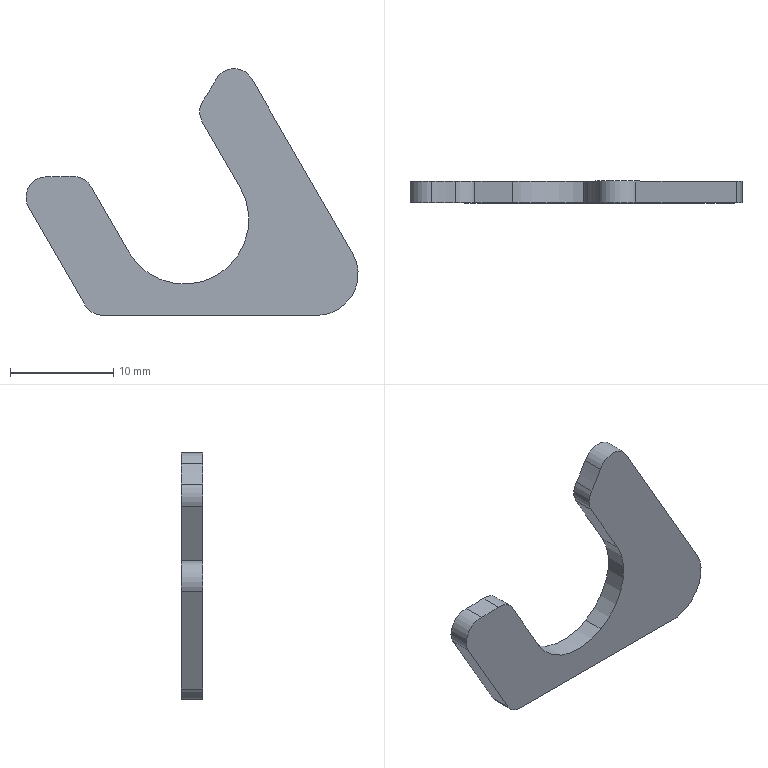Part | SolidWorks | features BaseBody 1 | 1 solid | 18 faces | box 32.238 x 2.1 x 23.947 mm | volume 666.378 mm3 | cylinder 11 | plane 7 | commonest cylinder face diameters 4 x5 8 x2 12.5 x2 35 x2
STEP:
#1=CARTESIAN_POINT('',(182.361,160.,-32.991));
#2=VERTEX_POINT('',#1);
#3=CARTESIAN_POINT('',(183.825,160.,-27.527));
#4=VERTEX_POINT('',#3);
#5=CARTESIAN_POINT('',(180.361,160.,-29.527));
#6=DIRECTION('',(0.,-1.,0.));
#7=DIRECTION('',(0.5,0.,-0.866));
#8=AXIS2_PLACEMENT_3D('',#5,#6,#7);
#9=CIRCLE('',#8,4.);
#10=EDGE_CURVE('',#2,#4,#9,.T.);
#11=ORIENTED_EDGE('',*,*,#10,.F.);
#12=CARTESIAN_POINT('',(182.361,162.1,-32.991));
#13=VERTEX_POINT('',#12);
#14=CARTESIAN_POINT('',(182.361,160.,-32.991));
#15=DIRECTION('',(0.,1.,0.));
#16=VECTOR('',#15,1000.);
#17=LINE('',#14,#16);
#18=EDGE_CURVE('',#2,#13,#17,.T.);
#19=ORIENTED_EDGE('',*,*,#18,.T.);
#20=CARTESIAN_POINT('',(183.825,162.1,-27.527));
#21=VERTEX_POINT('',#20);
#22=CARTESIAN_POINT('',(180.361,162.1,-29.527));
#23=DIRECTION('',(0.,-1.,0.));
#24=DIRECTION('',(0.5,0.,-0.866));
#25=AXIS2_PLACEMENT_3D('',#22,#23,#24);
#26=CIRCLE('',#25,4.);
#27=EDGE_CURVE('',#13,#21,#26,.T.);
#28=ORIENTED_EDGE('',*,*,#27,.T.);
#29=CARTESIAN_POINT('',(183.825,160.,-27.527));
#30=DIRECTION('',(0.,1.,0.));
#31=VECTOR('',#30,1000.);
#32=LINE('',#29,#31);
#33=EDGE_CURVE('',#4,#21,#32,.T.);
#34=ORIENTED_EDGE('',*,*,#33,.F.);
#35=EDGE_LOOP('',(#11,#19,#28,#34));
#36=FACE_OUTER_BOUND('',#35,.T.);
#37=CARTESIAN_POINT('',(180.361,160.,-29.527));
#38=DIRECTION('',(0.,1.,0.));
#39=DIRECTION('',(0.5,0.,-0.866));
#40=AXIS2_PLACEMENT_3D('',#37,#38,#39);
#41=CYLINDRICAL_SURFACE('',#40,4.);
#42=ADVANCED_FACE('',(#36),#41,.T.);
#43=CARTESIAN_POINT('',(170.625,160.,-29.663));
#44=VERTEX_POINT('',#43);
#45=CARTESIAN_POINT('',(162.087,160.,-27.375));
#46=VERTEX_POINT('',#45);
#47=CARTESIAN_POINT('',(167.5,160.,-24.25));
#48=DIRECTION('',(0.,1.,0.));
#49=DIRECTION('',(-0.5,0.,0.866));
#50=AXIS2_PLACEMENT_3D('',#47,#48,#49);
#51=CIRCLE('',#50,6.25);
#52=EDGE_CURVE('',#44,#46,#51,.T.);
#53=ORIENTED_EDGE('',*,*,#52,.F.);
#54=CARTESIAN_POINT('',(170.625,162.1,-29.663));
#55=VERTEX_POINT('',#54);
#56=CARTESIAN_POINT('',(170.625,160.,-29.663));
#57=DIRECTION('',(0.,1.,0.));
#58=VECTOR('',#57,1000.);
#59=LINE('',#56,#58);
#60=EDGE_CURVE('',#44,#55,#59,.T.);
#61=ORIENTED_EDGE('',*,*,#60,.T.);
#62=CARTESIAN_POINT('',(162.087,162.1,-27.375));
#63=VERTEX_POINT('',#62);
#64=CARTESIAN_POINT('',(167.5,162.1,-24.25));
#65=DIRECTION('',(0.,1.,0.));
#66=DIRECTION('',(-0.5,0.,0.866));
#67=AXIS2_PLACEMENT_3D('',#64,#65,#66);
#68=CIRCLE('',#67,6.25);
#69=EDGE_CURVE('',#55,#63,#68,.T.);
#70=ORIENTED_EDGE('',*,*,#69,.T.);
#71=CARTESIAN_POINT('',(162.087,160.,-27.375));
#72=DIRECTION('',(0.,1.,0.));
#73=VECTOR('',#72,1000.);
#74=LINE('',#71,#73);
#75=EDGE_CURVE('',#46,#63,#74,.T.);
#76=ORIENTED_EDGE('',*,*,#75,.F.);
#77=EDGE_LOOP('',(#53,#61,#70,#76));
#78=FACE_OUTER_BOUND('',#77,.T.);
#79=CARTESIAN_POINT('',(167.5,160.,-24.25));
#80=DIRECTION('',(0.,1.,0.));
#81=DIRECTION('',(0.5,0.,-0.866));
#82=AXIS2_PLACEMENT_3D('',#79,#80,#81);
#83=CYLINDRICAL_SURFACE('',#82,6.25);
#84=ADVANCED_FACE('',(#78),#83,.F.);
#85=ORIENTED_EDGE('',*,*,#60,.F.);
#86=CARTESIAN_POINT('',(172.913,160.,-21.125));
#87=VERTEX_POINT('',#86);
#88=CARTESIAN_POINT('',(167.5,160.,-24.25));
#89=DIRECTION('',(0.,1.,0.));
#90=DIRECTION('',(-0.5,0.,0.866));
#91=AXIS2_PLACEMENT_3D('',#88,#89,#90);
#92=CIRCLE('',#91,6.25);
#93=EDGE_CURVE('',#87,#44,#92,.T.);
#94=ORIENTED_EDGE('',*,*,#93,.F.);
#95=CARTESIAN_POINT('',(172.913,162.1,-21.125));
#96=VERTEX_POINT('',#95);
#97=CARTESIAN_POINT('',(172.913,160.,-21.125));
#98=DIRECTION('',(0.,1.,0.));
#99=VECTOR('',#98,1000.);
#100=LINE('',#97,#99);
#101=EDGE_CURVE('',#87,#96,#100,.T.);
#102=ORIENTED_EDGE('',*,*,#101,.T.);
#103=CARTESIAN_POINT('',(167.5,162.1,-24.25));
#104=DIRECTION('',(0.,1.,0.));
#105=DIRECTION('',(-0.5,0.,0.866));
#106=AXIS2_PLACEMENT_3D('',#103,#104,#105);
#107=CIRCLE('',#106,6.25);
#108=EDGE_CURVE('',#96,#55,#107,.T.);
#109=ORIENTED_EDGE('',*,*,#108,.T.);
#110=EDGE_LOOP('',(#85,#94,#102,#109));
#111=FACE_OUTER_BOUND('',#110,.T.);
#112=CARTESIAN_POINT('',(167.5,160.,-24.25));
#113=DIRECTION('',(0.,1.,0.));
#114=DIRECTION('',(0.5,0.,-0.866));
#115=AXIS2_PLACEMENT_3D('',#112,#113,#114);
#116=CYLINDRICAL_SURFACE('',#115,6.25);
#117=ADVANCED_FACE('',(#111),#116,.F.);
#118=CARTESIAN_POINT('',(158.422,162.1,-21.026));
#119=VERTEX_POINT('',#118);
#120=CARTESIAN_POINT('',(162.087,162.1,-27.375));
#121=DIRECTION('',(-0.5,0.,0.866));
#122=VECTOR('',#121,1000.);
#123=LINE('',#120,#122);
#124=EDGE_CURVE('',#63,#119,#123,.T.);
#125=ORIENTED_EDGE('',*,*,#124,.T.);
#126=CARTESIAN_POINT('',(158.422,160.,-21.026));
#127=VERTEX_POINT('',#126);
#128=CARTESIAN_POINT('',(158.422,160.,-21.026));
#129=DIRECTION('',(0.,1.,0.));
#130=VECTOR('',#129,1000.);
#131=LINE('',#128,#130);
#132=EDGE_CURVE('',#127,#119,#131,.T.);
#133=ORIENTED_EDGE('',*,*,#132,.F.);
#134=CARTESIAN_POINT('',(162.087,160.,-27.375));
#135=DIRECTION('',(-0.5,0.,0.866));
#136=VECTOR('',#135,1000.);
#137=LINE('',#134,#136);
#138=EDGE_CURVE('',#46,#127,#137,.T.);
#139=ORIENTED_EDGE('',*,*,#138,.F.);
#140=ORIENTED_EDGE('',*,*,#75,.T.);
#141=EDGE_LOOP('',(#125,#133,#139,#140));
#142=FACE_OUTER_BOUND('',#141,.T.);
#143=CARTESIAN_POINT('',(162.087,160.,-27.375));
#144=DIRECTION('',(-0.866,0.,-0.5));
#145=DIRECTION('',(0.5,0.,-0.866));
#146=AXIS2_PLACEMENT_3D('',#143,#144,#145);
#147=PLANE('',#146);
#148=ADVANCED_FACE('',(#142),#147,.F.);
#149=CARTESIAN_POINT('',(156.516,162.1,-20.033));
#150=VERTEX_POINT('',#149);
#151=CARTESIAN_POINT('',(156.69,162.1,-22.026));
#152=DIRECTION('',(0.,-1.,0.));
#153=DIRECTION('',(-0.5,0.,0.866));
#154=AXIS2_PLACEMENT_3D('',#151,#152,#153);
#155=CIRCLE('',#154,2.);
#156=EDGE_CURVE('',#119,#150,#155,.T.);
#157=ORIENTED_EDGE('',*,*,#156,.T.);
#158=CARTESIAN_POINT('',(156.516,160.,-20.033));
#159=VERTEX_POINT('',#158);
#160=CARTESIAN_POINT('',(156.516,160.,-20.033));
#161=DIRECTION('',(0.,1.,0.));
#162=VECTOR('',#161,1000.);
#163=LINE('',#160,#162);
#164=EDGE_CURVE('',#159,#150,#163,.T.);
#165=ORIENTED_EDGE('',*,*,#164,.F.);
#166=CARTESIAN_POINT('',(156.69,160.,-22.026));
#167=DIRECTION('',(0.,-1.,0.));
#168=DIRECTION('',(-0.5,0.,0.866));
#169=AXIS2_PLACEMENT_3D('',#166,#167,#168);
#170=CIRCLE('',#169,2.);
#171=EDGE_CURVE('',#127,#159,#170,.T.);
#172=ORIENTED_EDGE('',*,*,#171,.F.);
#173=ORIENTED_EDGE('',*,*,#132,.T.);
#174=EDGE_LOOP('',(#157,#165,#172,#173));
#175=FACE_OUTER_BOUND('',#174,.T.);
#176=CARTESIAN_POINT('',(156.69,160.,-22.026));
#177=DIRECTION('',(0.,1.,0.));
#178=DIRECTION('',(0.5,0.,-0.866));
#179=AXIS2_PLACEMENT_3D('',#176,#177,#178);
#180=CYLINDRICAL_SURFACE('',#179,2.);
#181=ADVANCED_FACE('',(#175),#180,.T.);
#182=CARTESIAN_POINT('',(154.213,162.1,-20.081));
#183=VERTEX_POINT('',#182);
#184=CARTESIAN_POINT('',(155.,162.1,-2.599));
#185=DIRECTION('',(0.,1.,0.));
#186=DIRECTION('',(-0.5,0.,0.866));
#187=AXIS2_PLACEMENT_3D('',#184,#185,#186);
#188=CIRCLE('',#187,17.5);
#189=EDGE_CURVE('',#150,#183,#188,.T.);
#190=ORIENTED_EDGE('',*,*,#189,.T.);
#191=CARTESIAN_POINT('',(154.213,160.,-20.081));
#192=VERTEX_POINT('',#191);
#193=CARTESIAN_POINT('',(154.213,160.,-20.081));
#194=DIRECTION('',(0.,1.,0.));
#195=VECTOR('',#194,1000.);
#196=LINE('',#193,#195);
#197=EDGE_CURVE('',#192,#183,#196,.T.);
#198=ORIENTED_EDGE('',*,*,#197,.F.);
#199=CARTESIAN_POINT('',(155.,160.,-2.599));
#200=DIRECTION('',(0.,1.,0.));
#201=DIRECTION('',(-0.5,0.,0.866));
#202=AXIS2_PLACEMENT_3D('',#199,#200,#201);
#203=CIRCLE('',#202,17.5);
#204=EDGE_CURVE('',#159,#192,#203,.T.);
#205=ORIENTED_EDGE('',*,*,#204,.F.);
#206=ORIENTED_EDGE('',*,*,#164,.T.);
#207=EDGE_LOOP('',(#190,#198,#205,#206));
#208=FACE_OUTER_BOUND('',#207,.T.);
#209=CARTESIAN_POINT('',(155.,160.,-2.599));
#210=DIRECTION('',(0.,1.,0.));
#211=DIRECTION('',(0.5,0.,-0.866));
#212=AXIS2_PLACEMENT_3D('',#209,#210,#211);
#213=CYLINDRICAL_SURFACE('',#212,17.5);
#214=ADVANCED_FACE('',(#208),#213,.F.);
#215=CARTESIAN_POINT('',(152.391,162.1,-23.079));
#216=VERTEX_POINT('',#215);
#217=CARTESIAN_POINT('',(154.123,162.1,-22.079));
#218=DIRECTION('',(0.,-1.,0.));
#219=DIRECTION('',(0.5,0.,-0.866));
#220=AXIS2_PLACEMENT_3D('',#217,#218,#219);
#221=CIRCLE('',#220,2.);
#222=EDGE_CURVE('',#183,#216,#221,.T.);
#223=ORIENTED_EDGE('',*,*,#222,.T.);
#224=CARTESIAN_POINT('',(152.391,160.,-23.079));
#225=VERTEX_POINT('',#224);
#226=CARTESIAN_POINT('',(152.391,160.,-23.079));
#227=DIRECTION('',(0.,1.,0.));
#228=VECTOR('',#227,1000.);
#229=LINE('',#226,#228);
#230=EDGE_CURVE('',#225,#216,#229,.T.);
#231=ORIENTED_EDGE('',*,*,#230,.F.);
#232=CARTESIAN_POINT('',(154.123,160.,-22.079));
#233=DIRECTION('',(0.,-1.,0.));
#234=DIRECTION('',(0.5,0.,-0.866));
#235=AXIS2_PLACEMENT_3D('',#232,#233,#234);
#236=CIRCLE('',#235,2.);
#237=EDGE_CURVE('',#192,#225,#236,.T.);
#238=ORIENTED_EDGE('',*,*,#237,.F.);
#239=ORIENTED_EDGE('',*,*,#197,.T.);
#240=EDGE_LOOP('',(#223,#231,#238,#239));
#241=FACE_OUTER_BOUND('',#240,.T.);
#242=CARTESIAN_POINT('',(154.123,160.,-22.079));
#243=DIRECTION('',(0.,1.,0.));
#244=DIRECTION('',(0.5,0.,-0.866));
#245=AXIS2_PLACEMENT_3D('',#242,#243,#244);
#246=CYLINDRICAL_SURFACE('',#245,2.);
#247=ADVANCED_FACE('',(#241),#246,.T.);
#248=CARTESIAN_POINT('',(157.844,162.1,-32.526));
#249=VERTEX_POINT('',#248);
#250=CARTESIAN_POINT('',(157.844,162.1,-32.526));
#251=DIRECTION('',(0.5,0.,-0.866));
#252=VECTOR('',#251,1000.);
#253=LINE('',#250,#252);
#254=EDGE_CURVE('',#216,#249,#253,.T.);
#255=ORIENTED_EDGE('',*,*,#254,.T.);
#256=CARTESIAN_POINT('',(157.844,160.,-32.526));
#257=VERTEX_POINT('',#256);
#258=CARTESIAN_POINT('',(157.844,160.,-32.526));
#259=DIRECTION('',(0.,1.,0.));
#260=VECTOR('',#259,1000.);
#261=LINE('',#258,#260);
#262=EDGE_CURVE('',#257,#249,#261,.T.);
#263=ORIENTED_EDGE('',*,*,#262,.F.);
#264=CARTESIAN_POINT('',(157.844,160.,-32.526));
#265=DIRECTION('',(0.5,0.,-0.866));
#266=VECTOR('',#265,1000.);
#267=LINE('',#264,#266);
#268=EDGE_CURVE('',#225,#257,#267,.T.);
#269=ORIENTED_EDGE('',*,*,#268,.F.);
#270=ORIENTED_EDGE('',*,*,#230,.T.);
#271=EDGE_LOOP('',(#255,#263,#269,#270));
#272=FACE_OUTER_BOUND('',#271,.T.);
#273=CARTESIAN_POINT('',(157.844,160.,-32.526));
#274=DIRECTION('',(0.866,0.,0.5));
#275=DIRECTION('',(-0.5,0.,0.866));
#276=AXIS2_PLACEMENT_3D('',#273,#274,#275);
#277=PLANE('',#276);
#278=ADVANCED_FACE('',(#272),#277,.F.);
#279=CARTESIAN_POINT('',(159.576,162.1,-33.526));
#280=VERTEX_POINT('',#279);
#281=CARTESIAN_POINT('',(159.576,162.1,-31.526));
#282=DIRECTION('',(0.,-1.,0.));
#283=DIRECTION('',(0.5,0.,-0.866));
#284=AXIS2_PLACEMENT_3D('',#281,#282,#283);
#285=CIRCLE('',#284,2.);
#286=EDGE_CURVE('',#249,#280,#285,.T.);
#287=ORIENTED_EDGE('',*,*,#286,.T.);
#288=CARTESIAN_POINT('',(159.576,160.,-33.526));
#289=VERTEX_POINT('',#288);
#290=CARTESIAN_POINT('',(159.576,160.,-33.526));
#291=DIRECTION('',(0.,1.,0.));
#292=VECTOR('',#291,1000.);
#293=LINE('',#290,#292);
#294=EDGE_CURVE('',#289,#280,#293,.T.);
#295=ORIENTED_EDGE('',*,*,#294,.F.);
#296=CARTESIAN_POINT('',(159.576,160.,-31.526));
#297=DIRECTION('',(0.,-1.,0.));
#298=DIRECTION('',(0.5,0.,-0.866));
#299=AXIS2_PLACEMENT_3D('',#296,#297,#298);
#300=CIRCLE('',#299,2.);
#301=EDGE_CURVE('',#257,#289,#300,.T.);
#302=ORIENTED_EDGE('',*,*,#301,.F.);
#303=ORIENTED_EDGE('',*,*,#262,.T.);
#304=EDGE_LOOP('',(#287,#295,#302,#303));
#305=FACE_OUTER_BOUND('',#304,.T.);
#306=CARTESIAN_POINT('',(159.576,160.,-31.526));
#307=DIRECTION('',(0.,1.,0.));
#308=DIRECTION('',(0.5,0.,-0.866));
#309=AXIS2_PLACEMENT_3D('',#306,#307,#308);
#310=CYLINDRICAL_SURFACE('',#309,2.);
#311=ADVANCED_FACE('',(#305),#310,.T.);
#312=CARTESIAN_POINT('',(180.361,162.1,-33.527));
#313=VERTEX_POINT('',#312);
#314=CARTESIAN_POINT('',(159.576,162.1,-33.526));
#315=DIRECTION('',(1.,0.,-0.00002301));
#316=VECTOR('',#315,1000.);
#317=LINE('',#314,#316);
#318=EDGE_CURVE('',#280,#313,#317,.T.);
#319=ORIENTED_EDGE('',*,*,#318,.T.);
#320=CARTESIAN_POINT('',(180.361,160.,-33.527));
#321=VERTEX_POINT('',#320);
#322=CARTESIAN_POINT('',(180.361,160.,-33.527));
#323=DIRECTION('',(0.,1.,0.));
#324=VECTOR('',#323,1000.);
#325=LINE('',#322,#324);
#326=EDGE_CURVE('',#321,#313,#325,.T.);
#327=ORIENTED_EDGE('',*,*,#326,.F.);
#328=CARTESIAN_POINT('',(159.576,160.,-33.526));
#329=DIRECTION('',(1.,0.,-0.00002301));
#330=VECTOR('',#329,1000.);
#331=LINE('',#328,#330);
#332=EDGE_CURVE('',#289,#321,#331,.T.);
#333=ORIENTED_EDGE('',*,*,#332,.F.);
#334=ORIENTED_EDGE('',*,*,#294,.T.);
#335=EDGE_LOOP('',(#319,#327,#333,#334));
#336=FACE_OUTER_BOUND('',#335,.T.);
#337=CARTESIAN_POINT('',(159.576,160.,-33.526));
#338=DIRECTION('',(0.00002301,0.,1.));
#339=DIRECTION('',(-1.,0.,0.00002301));
#340=AXIS2_PLACEMENT_3D('',#337,#338,#339);
#341=PLANE('',#340);
#342=ADVANCED_FACE('',(#336),#341,.F.);
#343=ORIENTED_EDGE('',*,*,#18,.F.);
#344=CARTESIAN_POINT('',(180.361,160.,-29.527));
#345=DIRECTION('',(0.,-1.,0.));
#346=DIRECTION('',(0.5,0.,-0.866));
#347=AXIS2_PLACEMENT_3D('',#344,#345,#346);
#348=CIRCLE('',#347,4.);
#349=EDGE_CURVE('',#321,#2,#348,.T.);
#350=ORIENTED_EDGE('',*,*,#349,.F.);
#351=ORIENTED_EDGE('',*,*,#326,.T.);
#352=CARTESIAN_POINT('',(180.361,162.1,-29.527));
#353=DIRECTION('',(0.,-1.,0.));
#354=DIRECTION('',(0.5,0.,-0.866));
#355=AXIS2_PLACEMENT_3D('',#352,#353,#354);
#356=CIRCLE('',#355,4.);
#357=EDGE_CURVE('',#313,#13,#356,.T.);
#358=ORIENTED_EDGE('',*,*,#357,.T.);
#359=EDGE_LOOP('',(#343,#350,#351,#358));
#360=FACE_OUTER_BOUND('',#359,.T.);
#361=CARTESIAN_POINT('',(180.361,160.,-29.527));
#362=DIRECTION('',(0.,1.,0.));
#363=DIRECTION('',(0.5,0.,-0.866));
#364=AXIS2_PLACEMENT_3D('',#361,#362,#363);
#365=CYLINDRICAL_SURFACE('',#364,4.);
#366=ADVANCED_FACE('',(#360),#365,.T.);
#367=CARTESIAN_POINT('',(174.041,162.1,-10.58));
#368=VERTEX_POINT('',#367);
#369=CARTESIAN_POINT('',(183.825,162.1,-27.527));
#370=DIRECTION('',(-0.5,0.,0.866));
#371=VECTOR('',#370,1000.);
#372=LINE('',#369,#371);
#373=EDGE_CURVE('',#21,#368,#372,.T.);
#374=ORIENTED_EDGE('',*,*,#373,.T.);
#375=CARTESIAN_POINT('',(174.041,160.,-10.58));
#376=VERTEX_POINT('',#375);
#377=CARTESIAN_POINT('',(174.041,160.,-10.58));
#378=DIRECTION('',(0.,1.,0.));
#379=VECTOR('',#378,1000.);
#380=LINE('',#377,#379);
#381=EDGE_CURVE('',#376,#368,#380,.T.);
#382=ORIENTED_EDGE('',*,*,#381,.F.);
#383=CARTESIAN_POINT('',(183.825,160.,-27.527));
#384=DIRECTION('',(-0.5,0.,0.866));
#385=VECTOR('',#384,1000.);
#386=LINE('',#383,#385);
#387=EDGE_CURVE('',#4,#376,#386,.T.);
#388=ORIENTED_EDGE('',*,*,#387,.F.);
#389=ORIENTED_EDGE('',*,*,#33,.T.);
#390=EDGE_LOOP('',(#374,#382,#388,#389));
#391=FACE_OUTER_BOUND('',#390,.T.);
#392=CARTESIAN_POINT('',(183.825,160.,-27.527));
#393=DIRECTION('',(-0.866,0.,-0.5));
#394=DIRECTION('',(0.5,0.,-0.866));
#395=AXIS2_PLACEMENT_3D('',#392,#393,#394);
#396=PLANE('',#395);
#397=ADVANCED_FACE('',(#391),#396,.F.);
#398=CARTESIAN_POINT('',(170.534,162.1,-10.659));
#399=VERTEX_POINT('',#398);
#400=CARTESIAN_POINT('',(172.309,162.1,-11.58));
#401=DIRECTION('',(0.,-1.,0.));
#402=DIRECTION('',(-0.5,0.,0.866));
#403=AXIS2_PLACEMENT_3D('',#400,#401,#402);
#404=CIRCLE('',#403,2.);
#405=EDGE_CURVE('',#368,#399,#404,.T.);
#406=ORIENTED_EDGE('',*,*,#405,.T.);
#407=CARTESIAN_POINT('',(170.534,160.,-10.659));
#408=VERTEX_POINT('',#407);
#409=CARTESIAN_POINT('',(170.534,160.,-10.659));
#410=DIRECTION('',(0.,1.,0.));
#411=VECTOR('',#410,1000.);
#412=LINE('',#409,#411);
#413=EDGE_CURVE('',#408,#399,#412,.T.);
#414=ORIENTED_EDGE('',*,*,#413,.F.);
#415=CARTESIAN_POINT('',(172.309,160.,-11.58));
#416=DIRECTION('',(0.,-1.,0.));
#417=DIRECTION('',(-0.5,0.,0.866));
#418=AXIS2_PLACEMENT_3D('',#415,#416,#417);
#419=CIRCLE('',#418,2.);
#420=EDGE_CURVE('',#376,#408,#419,.T.);
#421=ORIENTED_EDGE('',*,*,#420,.F.);
#422=ORIENTED_EDGE('',*,*,#381,.T.);
#423=EDGE_LOOP('',(#406,#414,#421,#422));
#424=FACE_OUTER_BOUND('',#423,.T.);
#425=CARTESIAN_POINT('',(172.309,160.,-11.58));
#426=DIRECTION('',(0.,1.,0.));
#427=DIRECTION('',(0.5,0.,-0.866));
#428=AXIS2_PLACEMENT_3D('',#425,#426,#427);
#429=CYLINDRICAL_SURFACE('',#428,2.);
#430=ADVANCED_FACE('',(#424),#429,.T.);
#431=CARTESIAN_POINT('',(169.341,162.1,-12.63));
#432=VERTEX_POINT('',#431);
#433=CARTESIAN_POINT('',(155.,162.1,-2.599));
#434=DIRECTION('',(0.,1.,0.));
#435=DIRECTION('',(-0.5,0.,0.866));
#436=AXIS2_PLACEMENT_3D('',#433,#434,#435);
#437=CIRCLE('',#436,17.5);
#438=EDGE_CURVE('',#399,#432,#437,.T.);
#439=ORIENTED_EDGE('',*,*,#438,.T.);
#440=CARTESIAN_POINT('',(169.341,160.,-12.63));
#441=VERTEX_POINT('',#440);
#442=CARTESIAN_POINT('',(169.341,160.,-12.63));
#443=DIRECTION('',(0.,1.,0.));
#444=VECTOR('',#443,1000.);
#445=LINE('',#442,#444);
#446=EDGE_CURVE('',#441,#432,#445,.T.);
#447=ORIENTED_EDGE('',*,*,#446,.F.);
#448=CARTESIAN_POINT('',(155.,160.,-2.599));
#449=DIRECTION('',(0.,1.,0.));
#450=DIRECTION('',(-0.5,0.,0.866));
#451=AXIS2_PLACEMENT_3D('',#448,#449,#450);
#452=CIRCLE('',#451,17.5);
#453=EDGE_CURVE('',#408,#441,#452,.T.);
#454=ORIENTED_EDGE('',*,*,#453,.F.);
#455=ORIENTED_EDGE('',*,*,#413,.T.);
#456=EDGE_LOOP('',(#439,#447,#454,#455));
#457=FACE_OUTER_BOUND('',#456,.T.);
#458=CARTESIAN_POINT('',(155.,160.,-2.599));
#459=DIRECTION('',(0.,1.,0.));
#460=DIRECTION('',(0.5,0.,-0.866));
#461=AXIS2_PLACEMENT_3D('',#458,#459,#460);
#462=CYLINDRICAL_SURFACE('',#461,17.5);
#463=ADVANCED_FACE('',(#457),#462,.F.);
#464=CARTESIAN_POINT('',(169.247,162.1,-14.776));
#465=VERTEX_POINT('',#464);
#466=CARTESIAN_POINT('',(170.979,162.1,-13.776));
#467=DIRECTION('',(0.,-1.,0.));
#468=DIRECTION('',(0.5,0.,-0.866));
#469=AXIS2_PLACEMENT_3D('',#466,#467,#468);
#470=CIRCLE('',#469,2.);
#471=EDGE_CURVE('',#432,#465,#470,.T.);
#472=ORIENTED_EDGE('',*,*,#471,.T.);
#473=CARTESIAN_POINT('',(169.247,160.,-14.776));
#474=VERTEX_POINT('',#473);
#475=CARTESIAN_POINT('',(169.247,160.,-14.776));
#476=DIRECTION('',(0.,1.,0.));
#477=VECTOR('',#476,1000.);
#478=LINE('',#475,#477);
#479=EDGE_CURVE('',#474,#465,#478,.T.);
#480=ORIENTED_EDGE('',*,*,#479,.F.);
#481=CARTESIAN_POINT('',(170.979,160.,-13.776));
#482=DIRECTION('',(0.,-1.,0.));
#483=DIRECTION('',(0.5,0.,-0.866));
#484=AXIS2_PLACEMENT_3D('',#481,#482,#483);
#485=CIRCLE('',#484,2.);
#486=EDGE_CURVE('',#441,#474,#485,.T.);
#487=ORIENTED_EDGE('',*,*,#486,.F.);
#488=ORIENTED_EDGE('',*,*,#446,.T.);
#489=EDGE_LOOP('',(#472,#480,#487,#488));
#490=FACE_OUTER_BOUND('',#489,.T.);
#491=CARTESIAN_POINT('',(170.979,160.,-13.776));
#492=DIRECTION('',(0.,1.,0.));
#493=DIRECTION('',(0.5,0.,-0.866));
#494=AXIS2_PLACEMENT_3D('',#491,#492,#493);
#495=CYLINDRICAL_SURFACE('',#494,2.);
#496=ADVANCED_FACE('',(#490),#495,.T.);
#497=CARTESIAN_POINT('',(172.913,162.1,-21.125));
#498=DIRECTION('',(0.5,0.,-0.866));
#499=VECTOR('',#498,1000.);
#500=LINE('',#497,#499);
#501=EDGE_CURVE('',#465,#96,#500,.T.);
#502=ORIENTED_EDGE('',*,*,#501,.T.);
#503=ORIENTED_EDGE('',*,*,#101,.F.);
#504=CARTESIAN_POINT('',(172.913,160.,-21.125));
#505=DIRECTION('',(0.5,0.,-0.866));
#506=VECTOR('',#505,1000.);
#507=LINE('',#504,#506);
#508=EDGE_CURVE('',#474,#87,#507,.T.);
#509=ORIENTED_EDGE('',*,*,#508,.F.);
#510=ORIENTED_EDGE('',*,*,#479,.T.);
#511=EDGE_LOOP('',(#502,#503,#509,#510));
#512=FACE_OUTER_BOUND('',#511,.T.);
#513=CARTESIAN_POINT('',(172.913,160.,-21.125));
#514=DIRECTION('',(0.866,0.,0.5));
#515=DIRECTION('',(-0.5,0.,0.866));
#516=AXIS2_PLACEMENT_3D('',#513,#514,#515);
#517=PLANE('',#516);
#518=ADVANCED_FACE('',(#512),#517,.F.);
#519=ORIENTED_EDGE('',*,*,#93,.T.);
#520=ORIENTED_EDGE('',*,*,#52,.T.);
#521=ORIENTED_EDGE('',*,*,#138,.T.);
#522=ORIENTED_EDGE('',*,*,#171,.T.);
#523=ORIENTED_EDGE('',*,*,#204,.T.);
#524=ORIENTED_EDGE('',*,*,#237,.T.);
#525=ORIENTED_EDGE('',*,*,#268,.T.);
#526=ORIENTED_EDGE('',*,*,#301,.T.);
#527=ORIENTED_EDGE('',*,*,#332,.T.);
#528=ORIENTED_EDGE('',*,*,#349,.T.);
#529=ORIENTED_EDGE('',*,*,#10,.T.);
#530=ORIENTED_EDGE('',*,*,#387,.T.);
#531=ORIENTED_EDGE('',*,*,#420,.T.);
#532=ORIENTED_EDGE('',*,*,#453,.T.);
#533=ORIENTED_EDGE('',*,*,#486,.T.);
#534=ORIENTED_EDGE('',*,*,#508,.T.);
#535=EDGE_LOOP('',(#519,#520,#521,#522,#523,#524,#525,#526,#527,#528,#529,#530,#531,#532,#533,#534));
#536=FACE_OUTER_BOUND('',#535,.T.);
#537=CARTESIAN_POINT('',(167.5,160.,-24.25));
#538=DIRECTION('',(0.,-1.,0.));
#539=DIRECTION('',(-0.5,0.,0.866));
#540=AXIS2_PLACEMENT_3D('',#537,#538,#539);
#541=PLANE('',#540);
#542=ADVANCED_FACE('',(#536),#541,.T.);
#543=ORIENTED_EDGE('',*,*,#108,.F.);
#544=ORIENTED_EDGE('',*,*,#501,.F.);
#545=ORIENTED_EDGE('',*,*,#471,.F.);
#546=ORIENTED_EDGE('',*,*,#438,.F.);
#547=ORIENTED_EDGE('',*,*,#405,.F.);
#548=ORIENTED_EDGE('',*,*,#373,.F.);
#549=ORIENTED_EDGE('',*,*,#27,.F.);
#550=ORIENTED_EDGE('',*,*,#357,.F.);
#551=ORIENTED_EDGE('',*,*,#318,.F.);
#552=ORIENTED_EDGE('',*,*,#286,.F.);
#553=ORIENTED_EDGE('',*,*,#254,.F.);
#554=ORIENTED_EDGE('',*,*,#222,.F.);
#555=ORIENTED_EDGE('',*,*,#189,.F.);
#556=ORIENTED_EDGE('',*,*,#156,.F.);
#557=ORIENTED_EDGE('',*,*,#124,.F.);
#558=ORIENTED_EDGE('',*,*,#69,.F.);
#559=EDGE_LOOP('',(#543,#544,#545,#546,#547,#548,#549,#550,#551,#552,#553,#554,#555,#556,#557,#558));
#560=FACE_OUTER_BOUND('',#559,.T.);
#561=CARTESIAN_POINT('',(167.5,162.1,-24.25));
#562=DIRECTION('',(0.,-1.,0.));
#563=DIRECTION('',(-0.5,0.,0.866));
#564=AXIS2_PLACEMENT_3D('',#561,#562,#563);
#565=PLANE('',#564);
#566=ADVANCED_FACE('',(#560),#565,.F.);
#567=CLOSED_SHELL('',(#42,#84,#117,#148,#181,#214,#247,#278,#311,#342,#366,#397,#430,#463,#496,#518,#542,#566));
#568=MANIFOLD_SOLID_BREP('',#567);
#569=CARTESIAN_POINT('',(0.,0.,0.));
#570=DIRECTION('',(0.,0.,1.));
#571=DIRECTION('',(1.,0.,0.));
#572=AXIS2_PLACEMENT_3D('',#569,#570,#571);
#573=(LENGTH_UNIT()NAMED_UNIT(*)SI_UNIT(.MILLI.,.METRE.));
#574=UNCERTAINTY_MEASURE_WITH_UNIT(LENGTH_MEASURE(0.00001),#573,'','');
#575=(NAMED_UNIT(*)PLANE_ANGLE_UNIT()SI_UNIT($,.RADIAN.));
#576=(NAMED_UNIT(*)SI_UNIT($,.STERADIAN.)SOLID_ANGLE_UNIT());
#577=(GEOMETRIC_REPRESENTATION_CONTEXT(3)GLOBAL_UNCERTAINTY_ASSIGNED_CONTEXT((#574))GLOBAL_UNIT_ASSIGNED_CONTEXT((#573,#575,#576))REPRESENTATION_CONTEXT('',''));
#578=ADVANCED_BREP_SHAPE_REPRESENTATION('',(#568,#572),#577);